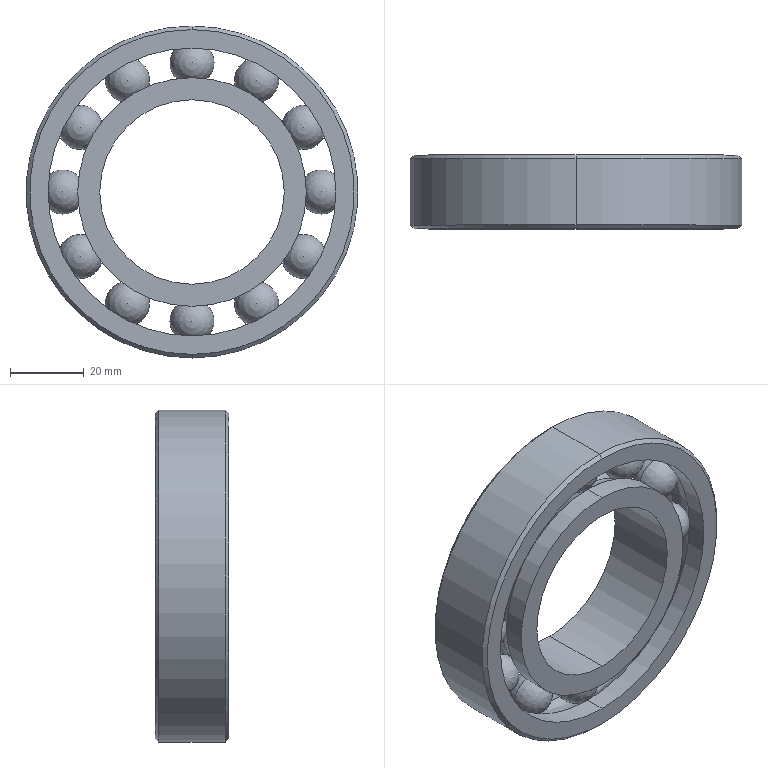Part | SolidWorks | features Revolution 13, Chamfer 1 | 14 solids | 50 faces | box 90 x 20 x 90 mm | volume 54381 mm3 | sphere 24 | cylinder 10 | torus 6 | cone 6 | plane 4 | commonest cylinder face diameters 62 x4 50 x2 78 x2 90 x2
STEP:
#1=CARTESIAN_POINT('',(0.,4.472,31.));
#2=VERTEX_POINT('',#1);
#3=CARTESIAN_POINT('',(0.,0.,29.));
#4=VERTEX_POINT('',#3);
#5=CARTESIAN_POINT('',(0.,0.,35.));
#6=DIRECTION('',(-1.,0.,0.));
#7=DIRECTION('',(0.,0.,1.));
#8=AXIS2_PLACEMENT_3D('',#5,#6,#7);
#9=CIRCLE('',#8,6.);
#10=EDGE_CURVE('',#2,#4,#9,.T.);
#11=ORIENTED_EDGE('',*,*,#10,.T.);
#12=CARTESIAN_POINT('',(0.,0.,-29.));
#13=VERTEX_POINT('',#12);
#14=CARTESIAN_POINT('',(0.,0.,0.));
#15=DIRECTION('',(0.,1.,0.));
#16=DIRECTION('',(0.,0.,1.));
#17=AXIS2_PLACEMENT_3D('',#14,#15,#16);
#18=CIRCLE('',#17,29.);
#19=EDGE_CURVE('',#4,#13,#18,.T.);
#20=ORIENTED_EDGE('',*,*,#19,.T.);
#21=CARTESIAN_POINT('',(0.,4.472,-31.));
#22=VERTEX_POINT('',#21);
#23=CARTESIAN_POINT('',(0.,0.,-35.));
#24=DIRECTION('',(1.,0.,0.));
#25=DIRECTION('',(0.,0.,-1.));
#26=AXIS2_PLACEMENT_3D('',#23,#24,#25);
#27=CIRCLE('',#26,6.);
#28=EDGE_CURVE('',#22,#13,#27,.T.);
#29=ORIENTED_EDGE('',*,*,#28,.F.);
#30=CARTESIAN_POINT('',(0.,4.472,0.));
#31=DIRECTION('',(0.,1.,0.));
#32=DIRECTION('',(0.,0.,1.));
#33=AXIS2_PLACEMENT_3D('',#30,#31,#32);
#34=CIRCLE('',#33,31.);
#35=EDGE_CURVE('',#2,#22,#34,.T.);
#36=ORIENTED_EDGE('',*,*,#35,.F.);
#37=EDGE_LOOP('',(#11,#20,#29,#36));
#38=FACE_OUTER_BOUND('',#37,.T.);
#39=CARTESIAN_POINT('',(0.,0.,0.));
#40=DIRECTION('',(0.,1.,0.));
#41=DIRECTION('',(0.,0.,1.));
#42=AXIS2_PLACEMENT_3D('',#39,#40,#41);
#43=TOROIDAL_SURFACE('',#42,35.,6.);
#44=ADVANCED_FACE('',(#38),#43,.F.);
#45=ORIENTED_EDGE('',*,*,#28,.T.);
#46=CARTESIAN_POINT('',(0.,0.,0.));
#47=DIRECTION('',(0.,1.,0.));
#48=DIRECTION('',(0.,0.,1.));
#49=AXIS2_PLACEMENT_3D('',#46,#47,#48);
#50=CIRCLE('',#49,29.);
#51=EDGE_CURVE('',#13,#4,#50,.T.);
#52=ORIENTED_EDGE('',*,*,#51,.T.);
#53=ORIENTED_EDGE('',*,*,#10,.F.);
#54=CARTESIAN_POINT('',(0.,4.472,0.));
#55=DIRECTION('',(0.,1.,0.));
#56=DIRECTION('',(0.,0.,1.));
#57=AXIS2_PLACEMENT_3D('',#54,#55,#56);
#58=CIRCLE('',#57,31.);
#59=EDGE_CURVE('',#22,#2,#58,.T.);
#60=ORIENTED_EDGE('',*,*,#59,.F.);
#61=EDGE_LOOP('',(#45,#52,#53,#60));
#62=FACE_OUTER_BOUND('',#61,.T.);
#63=CARTESIAN_POINT('',(0.,0.,0.));
#64=DIRECTION('',(0.,1.,0.));
#65=DIRECTION('',(0.,0.,1.));
#66=AXIS2_PLACEMENT_3D('',#63,#64,#65);
#67=TOROIDAL_SURFACE('',#66,35.,6.);
#68=ADVANCED_FACE('',(#62),#67,.F.);
#69=ORIENTED_EDGE('',*,*,#35,.T.);
#70=CARTESIAN_POINT('',(0.,10.,-31.));
#71=VERTEX_POINT('',#70);
#72=CARTESIAN_POINT('',(0.,0.,-31.));
#73=DIRECTION('',(0.,1.,0.));
#74=VECTOR('',#73,1000.);
#75=LINE('',#72,#74);
#76=EDGE_CURVE('',#22,#71,#75,.T.);
#77=ORIENTED_EDGE('',*,*,#76,.T.);
#78=CARTESIAN_POINT('',(0.,10.,31.));
#79=VERTEX_POINT('',#78);
#80=CARTESIAN_POINT('',(0.,10.,0.));
#81=DIRECTION('',(0.,1.,0.));
#82=DIRECTION('',(0.,0.,1.));
#83=AXIS2_PLACEMENT_3D('',#80,#81,#82);
#84=CIRCLE('',#83,31.);
#85=EDGE_CURVE('',#79,#71,#84,.T.);
#86=ORIENTED_EDGE('',*,*,#85,.F.);
#87=CARTESIAN_POINT('',(0.,0.,31.));
#88=DIRECTION('',(0.,1.,0.));
#89=VECTOR('',#88,1000.);
#90=LINE('',#87,#89);
#91=EDGE_CURVE('',#2,#79,#90,.T.);
#92=ORIENTED_EDGE('',*,*,#91,.F.);
#93=EDGE_LOOP('',(#69,#77,#86,#92));
#94=FACE_OUTER_BOUND('',#93,.T.);
#95=CARTESIAN_POINT('',(0.,0.,0.));
#96=DIRECTION('',(0.,1.,0.));
#97=DIRECTION('',(0.,0.,1.));
#98=AXIS2_PLACEMENT_3D('',#95,#96,#97);
#99=CYLINDRICAL_SURFACE('',#98,31.);
#100=ADVANCED_FACE('',(#94),#99,.T.);
#101=CARTESIAN_POINT('',(0.,-10.,-25.));
#102=VERTEX_POINT('',#101);
#103=CARTESIAN_POINT('',(0.,-10.,25.));
#104=VERTEX_POINT('',#103);
#105=CARTESIAN_POINT('',(0.,-10.,0.));
#106=DIRECTION('',(0.,1.,0.));
#107=DIRECTION('',(0.,0.,1.));
#108=AXIS2_PLACEMENT_3D('',#105,#106,#107);
#109=CIRCLE('',#108,25.);
#110=EDGE_CURVE('',#102,#104,#109,.T.);
#111=ORIENTED_EDGE('',*,*,#110,.F.);
#112=CARTESIAN_POINT('',(0.,10.,-25.));
#113=VERTEX_POINT('',#112);
#114=CARTESIAN_POINT('',(0.,0.,-25.));
#115=DIRECTION('',(0.,1.,0.));
#116=VECTOR('',#115,1000.);
#117=LINE('',#114,#116);
#118=EDGE_CURVE('',#102,#113,#117,.T.);
#119=ORIENTED_EDGE('',*,*,#118,.T.);
#120=CARTESIAN_POINT('',(0.,10.,25.));
#121=VERTEX_POINT('',#120);
#122=CARTESIAN_POINT('',(0.,10.,0.));
#123=DIRECTION('',(0.,1.,0.));
#124=DIRECTION('',(0.,0.,1.));
#125=AXIS2_PLACEMENT_3D('',#122,#123,#124);
#126=CIRCLE('',#125,25.);
#127=EDGE_CURVE('',#113,#121,#126,.T.);
#128=ORIENTED_EDGE('',*,*,#127,.T.);
#129=CARTESIAN_POINT('',(0.,0.,25.));
#130=DIRECTION('',(0.,1.,0.));
#131=VECTOR('',#130,1000.);
#132=LINE('',#129,#131);
#133=EDGE_CURVE('',#104,#121,#132,.T.);
#134=ORIENTED_EDGE('',*,*,#133,.F.);
#135=EDGE_LOOP('',(#111,#119,#128,#134));
#136=FACE_OUTER_BOUND('',#135,.T.);
#137=CARTESIAN_POINT('',(0.,0.,0.));
#138=DIRECTION('',(0.,1.,0.));
#139=DIRECTION('',(0.,0.,1.));
#140=AXIS2_PLACEMENT_3D('',#137,#138,#139);
#141=CYLINDRICAL_SURFACE('',#140,25.);
#142=ADVANCED_FACE('',(#136),#141,.F.);
#143=CARTESIAN_POINT('',(0.,-10.,31.));
#144=VERTEX_POINT('',#143);
#145=CARTESIAN_POINT('',(0.,-10.,-31.));
#146=VERTEX_POINT('',#145);
#147=CARTESIAN_POINT('',(0.,-10.,0.));
#148=DIRECTION('',(0.,1.,0.));
#149=DIRECTION('',(0.,0.,1.));
#150=AXIS2_PLACEMENT_3D('',#147,#148,#149);
#151=CIRCLE('',#150,31.);
#152=EDGE_CURVE('',#144,#146,#151,.T.);
#153=ORIENTED_EDGE('',*,*,#152,.T.);
#154=CARTESIAN_POINT('',(0.,-4.472,-31.));
#155=VERTEX_POINT('',#154);
#156=CARTESIAN_POINT('',(0.,0.,-31.));
#157=DIRECTION('',(0.,1.,0.));
#158=VECTOR('',#157,1000.);
#159=LINE('',#156,#158);
#160=EDGE_CURVE('',#146,#155,#159,.T.);
#161=ORIENTED_EDGE('',*,*,#160,.T.);
#162=CARTESIAN_POINT('',(0.,-4.472,31.));
#163=VERTEX_POINT('',#162);
#164=CARTESIAN_POINT('',(0.,-4.472,0.));
#165=DIRECTION('',(0.,1.,0.));
#166=DIRECTION('',(0.,0.,1.));
#167=AXIS2_PLACEMENT_3D('',#164,#165,#166);
#168=CIRCLE('',#167,31.);
#169=EDGE_CURVE('',#163,#155,#168,.T.);
#170=ORIENTED_EDGE('',*,*,#169,.F.);
#171=CARTESIAN_POINT('',(0.,0.,31.));
#172=DIRECTION('',(0.,1.,0.));
#173=VECTOR('',#172,1000.);
#174=LINE('',#171,#173);
#175=EDGE_CURVE('',#144,#163,#174,.T.);
#176=ORIENTED_EDGE('',*,*,#175,.F.);
#177=EDGE_LOOP('',(#153,#161,#170,#176));
#178=FACE_OUTER_BOUND('',#177,.T.);
#179=CARTESIAN_POINT('',(0.,0.,0.));
#180=DIRECTION('',(0.,1.,0.));
#181=DIRECTION('',(0.,0.,1.));
#182=AXIS2_PLACEMENT_3D('',#179,#180,#181);
#183=CYLINDRICAL_SURFACE('',#182,31.);
#184=ADVANCED_FACE('',(#178),#183,.T.);
#185=ORIENTED_EDGE('',*,*,#51,.F.);
#186=CARTESIAN_POINT('',(0.,0.,-35.));
#187=DIRECTION('',(1.,0.,0.));
#188=DIRECTION('',(0.,0.,-1.));
#189=AXIS2_PLACEMENT_3D('',#186,#187,#188);
#190=CIRCLE('',#189,6.);
#191=EDGE_CURVE('',#13,#155,#190,.T.);
#192=ORIENTED_EDGE('',*,*,#191,.T.);
#193=CARTESIAN_POINT('',(0.,-4.472,0.));
#194=DIRECTION('',(0.,1.,0.));
#195=DIRECTION('',(0.,0.,1.));
#196=AXIS2_PLACEMENT_3D('',#193,#194,#195);
#197=CIRCLE('',#196,31.);
#198=EDGE_CURVE('',#155,#163,#197,.T.);
#199=ORIENTED_EDGE('',*,*,#198,.T.);
#200=CARTESIAN_POINT('',(0.,0.,35.));
#201=DIRECTION('',(-1.,0.,0.));
#202=DIRECTION('',(0.,0.,1.));
#203=AXIS2_PLACEMENT_3D('',#200,#201,#202);
#204=CIRCLE('',#203,6.);
#205=EDGE_CURVE('',#4,#163,#204,.T.);
#206=ORIENTED_EDGE('',*,*,#205,.F.);
#207=EDGE_LOOP('',(#185,#192,#199,#206));
#208=FACE_OUTER_BOUND('',#207,.T.);
#209=CARTESIAN_POINT('',(0.,0.,0.));
#210=DIRECTION('',(0.,1.,0.));
#211=DIRECTION('',(0.,0.,1.));
#212=AXIS2_PLACEMENT_3D('',#209,#210,#211);
#213=TOROIDAL_SURFACE('',#212,35.,6.);
#214=ADVANCED_FACE('',(#208),#213,.F.);
#215=ORIENTED_EDGE('',*,*,#19,.F.);
#216=ORIENTED_EDGE('',*,*,#205,.T.);
#217=ORIENTED_EDGE('',*,*,#169,.T.);
#218=ORIENTED_EDGE('',*,*,#191,.F.);
#219=EDGE_LOOP('',(#215,#216,#217,#218));
#220=FACE_OUTER_BOUND('',#219,.T.);
#221=CARTESIAN_POINT('',(0.,0.,0.));
#222=DIRECTION('',(0.,1.,0.));
#223=DIRECTION('',(0.,0.,1.));
#224=AXIS2_PLACEMENT_3D('',#221,#222,#223);
#225=TOROIDAL_SURFACE('',#224,35.,6.);
#226=ADVANCED_FACE('',(#220),#225,.F.);
#227=ORIENTED_EDGE('',*,*,#160,.F.);
#228=CARTESIAN_POINT('',(0.,-10.,0.));
#229=DIRECTION('',(0.,1.,0.));
#230=DIRECTION('',(0.,0.,1.));
#231=AXIS2_PLACEMENT_3D('',#228,#229,#230);
#232=CIRCLE('',#231,31.);
#233=EDGE_CURVE('',#146,#144,#232,.T.);
#234=ORIENTED_EDGE('',*,*,#233,.T.);
#235=ORIENTED_EDGE('',*,*,#175,.T.);
#236=ORIENTED_EDGE('',*,*,#198,.F.);
#237=EDGE_LOOP('',(#227,#234,#235,#236));
#238=FACE_OUTER_BOUND('',#237,.T.);
#239=CARTESIAN_POINT('',(0.,0.,0.));
#240=DIRECTION('',(0.,1.,0.));
#241=DIRECTION('',(0.,0.,1.));
#242=AXIS2_PLACEMENT_3D('',#239,#240,#241);
#243=CYLINDRICAL_SURFACE('',#242,31.);
#244=ADVANCED_FACE('',(#238),#243,.T.);
#245=CARTESIAN_POINT('',(0.,-10.,0.));
#246=DIRECTION('',(0.,1.,0.));
#247=DIRECTION('',(0.,0.,1.));
#248=AXIS2_PLACEMENT_3D('',#245,#246,#247);
#249=CIRCLE('',#248,25.);
#250=EDGE_CURVE('',#104,#102,#249,.T.);
#251=ORIENTED_EDGE('',*,*,#250,.T.);
#252=ORIENTED_EDGE('',*,*,#110,.T.);
#253=EDGE_LOOP('',(#251,#252));
#254=FACE_BOUND('',#253,.T.);
#255=ORIENTED_EDGE('',*,*,#152,.F.);
#256=ORIENTED_EDGE('',*,*,#233,.F.);
#257=EDGE_LOOP('',(#255,#256));
#258=FACE_OUTER_BOUND('',#257,.T.);
#259=CARTESIAN_POINT('',(-25.,-10.,0.));
#260=DIRECTION('',(0.,-1.,0.));
#261=DIRECTION('',(0.,0.,-1.));
#262=AXIS2_PLACEMENT_3D('',#259,#260,#261);
#263=PLANE('',#262);
#264=ADVANCED_FACE('',(#254,#258),#263,.T.);
#265=ORIENTED_EDGE('',*,*,#118,.F.);
#266=ORIENTED_EDGE('',*,*,#250,.F.);
#267=ORIENTED_EDGE('',*,*,#133,.T.);
#268=CARTESIAN_POINT('',(0.,10.,0.));
#269=DIRECTION('',(0.,1.,0.));
#270=DIRECTION('',(0.,0.,1.));
#271=AXIS2_PLACEMENT_3D('',#268,#269,#270);
#272=CIRCLE('',#271,25.);
#273=EDGE_CURVE('',#121,#113,#272,.T.);
#274=ORIENTED_EDGE('',*,*,#273,.T.);
#275=EDGE_LOOP('',(#265,#266,#267,#274));
#276=FACE_OUTER_BOUND('',#275,.T.);
#277=CARTESIAN_POINT('',(0.,0.,0.));
#278=DIRECTION('',(0.,1.,0.));
#279=DIRECTION('',(0.,0.,1.));
#280=AXIS2_PLACEMENT_3D('',#277,#278,#279);
#281=CYLINDRICAL_SURFACE('',#280,25.);
#282=ADVANCED_FACE('',(#276),#281,.F.);
#283=ORIENTED_EDGE('',*,*,#85,.T.);
#284=CARTESIAN_POINT('',(0.,10.,0.));
#285=DIRECTION('',(0.,1.,0.));
#286=DIRECTION('',(0.,0.,1.));
#287=AXIS2_PLACEMENT_3D('',#284,#285,#286);
#288=CIRCLE('',#287,31.);
#289=EDGE_CURVE('',#71,#79,#288,.T.);
#290=ORIENTED_EDGE('',*,*,#289,.T.);
#291=EDGE_LOOP('',(#283,#290));
#292=FACE_OUTER_BOUND('',#291,.T.);
#293=ORIENTED_EDGE('',*,*,#273,.F.);
#294=ORIENTED_EDGE('',*,*,#127,.F.);
#295=EDGE_LOOP('',(#293,#294));
#296=FACE_BOUND('',#295,.T.);
#297=CARTESIAN_POINT('',(-25.,10.,0.));
#298=DIRECTION('',(0.,1.,0.));
#299=DIRECTION('',(0.,0.,1.));
#300=AXIS2_PLACEMENT_3D('',#297,#298,#299);
#301=PLANE('',#300);
#302=ADVANCED_FACE('',(#292,#296),#301,.T.);
#303=ORIENTED_EDGE('',*,*,#76,.F.);
#304=ORIENTED_EDGE('',*,*,#59,.T.);
#305=ORIENTED_EDGE('',*,*,#91,.T.);
#306=ORIENTED_EDGE('',*,*,#289,.F.);
#307=EDGE_LOOP('',(#303,#304,#305,#306));
#308=FACE_OUTER_BOUND('',#307,.T.);
#309=CARTESIAN_POINT('',(0.,0.,0.));
#310=DIRECTION('',(0.,1.,0.));
#311=DIRECTION('',(0.,0.,1.));
#312=AXIS2_PLACEMENT_3D('',#309,#310,#311);
#313=CYLINDRICAL_SURFACE('',#312,31.);
#314=ADVANCED_FACE('',(#308),#313,.T.);
#315=CLOSED_SHELL('',(#44,#68,#100,#142,#184,#214,#226,#244,#264,#282,#302,#314));
#316=MANIFOLD_SOLID_BREP('',#315);
#317=CARTESIAN_POINT('',(0.,-10.,-44.));
#318=VERTEX_POINT('',#317);
#319=CARTESIAN_POINT('',(0.,-10.,44.));
#320=VERTEX_POINT('',#319);
#321=CARTESIAN_POINT('',(0.,-10.,0.));
#322=DIRECTION('',(0.,-1.,0.));
#323=DIRECTION('',(0.,0.,-1.));
#324=AXIS2_PLACEMENT_3D('',#321,#322,#323);
#325=CIRCLE('',#324,44.);
#326=EDGE_CURVE('',#318,#320,#325,.T.);
#327=ORIENTED_EDGE('',*,*,#326,.F.);
#328=CARTESIAN_POINT('',(0.,-9.,-45.));
#329=VERTEX_POINT('',#328);
#330=CARTESIAN_POINT('',(0.,-9.,-45.));
#331=DIRECTION('',(0.,0.7071,-0.7071));
#332=VECTOR('',#331,1000.);
#333=LINE('',#330,#332);
#334=EDGE_CURVE('',#318,#329,#333,.T.);
#335=ORIENTED_EDGE('',*,*,#334,.T.);
#336=CARTESIAN_POINT('',(0.,-9.,45.));
#337=VERTEX_POINT('',#336);
#338=CARTESIAN_POINT('',(0.,-9.,0.));
#339=DIRECTION('',(0.,1.,0.));
#340=DIRECTION('',(0.,0.,-1.));
#341=AXIS2_PLACEMENT_3D('',#338,#339,#340);
#342=CIRCLE('',#341,45.);
#343=EDGE_CURVE('',#337,#329,#342,.T.);
#344=ORIENTED_EDGE('',*,*,#343,.F.);
#345=CARTESIAN_POINT('',(0.,-9.,45.));
#346=DIRECTION('',(0.,0.7071,0.7071));
#347=VECTOR('',#346,1000.);
#348=LINE('',#345,#347);
#349=EDGE_CURVE('',#320,#337,#348,.T.);
#350=ORIENTED_EDGE('',*,*,#349,.F.);
#351=EDGE_LOOP('',(#327,#335,#344,#350));
#352=FACE_OUTER_BOUND('',#351,.T.);
#353=CARTESIAN_POINT('',(0.,-9.,0.));
#354=DIRECTION('',(0.,1.,0.));
#355=DIRECTION('',(0.,0.,1.));
#356=AXIS2_PLACEMENT_3D('',#353,#354,#355);
#357=CONICAL_SURFACE('',#356,45.,0.7854);
#358=ADVANCED_FACE('',(#352),#357,.T.);
#359=CARTESIAN_POINT('',(0.,10.,44.));
#360=VERTEX_POINT('',#359);
#361=CARTESIAN_POINT('',(0.,10.,-44.));
#362=VERTEX_POINT('',#361);
#363=CARTESIAN_POINT('',(0.,10.,0.));
#364=DIRECTION('',(0.,1.,0.));
#365=DIRECTION('',(0.,0.,1.));
#366=AXIS2_PLACEMENT_3D('',#363,#364,#365);
#367=CIRCLE('',#366,44.);
#368=EDGE_CURVE('',#360,#362,#367,.T.);
#369=ORIENTED_EDGE('',*,*,#368,.F.);
#370=CARTESIAN_POINT('',(0.,9.,45.));
#371=VERTEX_POINT('',#370);
#372=CARTESIAN_POINT('',(0.,10.,44.));
#373=DIRECTION('',(0.,-0.7071,0.7071));
#374=VECTOR('',#373,1000.);
#375=LINE('',#372,#374);
#376=EDGE_CURVE('',#360,#371,#375,.T.);
#377=ORIENTED_EDGE('',*,*,#376,.T.);
#378=CARTESIAN_POINT('',(0.,9.,-45.));
#379=VERTEX_POINT('',#378);
#380=CARTESIAN_POINT('',(0.,9.,0.));
#381=DIRECTION('',(0.,-1.,0.));
#382=DIRECTION('',(0.,0.,1.));
#383=AXIS2_PLACEMENT_3D('',#380,#381,#382);
#384=CIRCLE('',#383,45.);
#385=EDGE_CURVE('',#379,#371,#384,.T.);
#386=ORIENTED_EDGE('',*,*,#385,.F.);
#387=CARTESIAN_POINT('',(0.,10.,-44.));
#388=DIRECTION('',(0.,-0.7071,-0.7071));
#389=VECTOR('',#388,1000.);
#390=LINE('',#387,#389);
#391=EDGE_CURVE('',#362,#379,#390,.T.);
#392=ORIENTED_EDGE('',*,*,#391,.F.);
#393=EDGE_LOOP('',(#369,#377,#386,#392));
#394=FACE_OUTER_BOUND('',#393,.T.);
#395=CARTESIAN_POINT('',(0.,10.,0.));
#396=DIRECTION('',(0.,-1.,0.));
#397=DIRECTION('',(0.,0.,-1.));
#398=AXIS2_PLACEMENT_3D('',#395,#396,#397);
#399=CONICAL_SURFACE('',#398,44.,0.7854);
#400=ADVANCED_FACE('',(#394),#399,.T.);
#401=CARTESIAN_POINT('',(0.,-10.,-39.));
#402=VERTEX_POINT('',#401);
#403=CARTESIAN_POINT('',(0.,-10.,39.));
#404=VERTEX_POINT('',#403);
#405=CARTESIAN_POINT('',(0.,-10.,0.));
#406=DIRECTION('',(0.,1.,0.));
#407=DIRECTION('',(0.,0.,1.));
#408=AXIS2_PLACEMENT_3D('',#405,#406,#407);
#409=CIRCLE('',#408,39.);
#410=EDGE_CURVE('',#402,#404,#409,.T.);
#411=ORIENTED_EDGE('',*,*,#410,.F.);
#412=CARTESIAN_POINT('',(0.,-4.472,-39.));
#413=VERTEX_POINT('',#412);
#414=CARTESIAN_POINT('',(0.,0.,-39.));
#415=DIRECTION('',(0.,1.,0.));
#416=VECTOR('',#415,1000.);
#417=LINE('',#414,#416);
#418=EDGE_CURVE('',#402,#413,#417,.T.);
#419=ORIENTED_EDGE('',*,*,#418,.T.);
#420=CARTESIAN_POINT('',(0.,-4.472,39.));
#421=VERTEX_POINT('',#420);
#422=CARTESIAN_POINT('',(0.,-4.472,0.));
#423=DIRECTION('',(0.,1.,0.));
#424=DIRECTION('',(0.,0.,1.));
#425=AXIS2_PLACEMENT_3D('',#422,#423,#424);
#426=CIRCLE('',#425,39.);
#427=EDGE_CURVE('',#413,#421,#426,.T.);
#428=ORIENTED_EDGE('',*,*,#427,.T.);
#429=CARTESIAN_POINT('',(0.,0.,39.));
#430=DIRECTION('',(0.,1.,0.));
#431=VECTOR('',#430,1000.);
#432=LINE('',#429,#431);
#433=EDGE_CURVE('',#404,#421,#432,.T.);
#434=ORIENTED_EDGE('',*,*,#433,.F.);
#435=EDGE_LOOP('',(#411,#419,#428,#434));
#436=FACE_OUTER_BOUND('',#435,.T.);
#437=CARTESIAN_POINT('',(0.,0.,0.));
#438=DIRECTION('',(0.,1.,0.));
#439=DIRECTION('',(0.,0.,1.));
#440=AXIS2_PLACEMENT_3D('',#437,#438,#439);
#441=CYLINDRICAL_SURFACE('',#440,39.);
#442=ADVANCED_FACE('',(#436),#441,.F.);
#443=ORIENTED_EDGE('',*,*,#343,.T.);
#444=CARTESIAN_POINT('',(0.,0.,-45.));
#445=DIRECTION('',(0.,1.,0.));
#446=VECTOR('',#445,1000.);
#447=LINE('',#444,#446);
#448=EDGE_CURVE('',#329,#379,#447,.T.);
#449=ORIENTED_EDGE('',*,*,#448,.T.);
#450=ORIENTED_EDGE('',*,*,#385,.T.);
#451=CARTESIAN_POINT('',(0.,0.,45.));
#452=DIRECTION('',(0.,1.,0.));
#453=VECTOR('',#452,1000.);
#454=LINE('',#451,#453);
#455=EDGE_CURVE('',#337,#371,#454,.T.);
#456=ORIENTED_EDGE('',*,*,#455,.F.);
#457=EDGE_LOOP('',(#443,#449,#450,#456));
#458=FACE_OUTER_BOUND('',#457,.T.);
#459=CARTESIAN_POINT('',(0.,0.,0.));
#460=DIRECTION('',(0.,1.,0.));
#461=DIRECTION('',(0.,0.,1.));
#462=AXIS2_PLACEMENT_3D('',#459,#460,#461);
#463=CYLINDRICAL_SURFACE('',#462,45.);
#464=ADVANCED_FACE('',(#458),#463,.T.);
#465=CARTESIAN_POINT('',(0.,3.,-40.196));
#466=VERTEX_POINT('',#465);
#467=CARTESIAN_POINT('',(0.,3.,40.196));
#468=VERTEX_POINT('',#467);
#469=CARTESIAN_POINT('',(0.,3.,0.));
#470=DIRECTION('',(0.,1.,0.));
#471=DIRECTION('',(0.,0.,1.));
#472=AXIS2_PLACEMENT_3D('',#469,#470,#471);
#473=CIRCLE('',#472,40.196);
#474=EDGE_CURVE('',#466,#468,#473,.T.);
#475=ORIENTED_EDGE('',*,*,#474,.F.);
#476=CARTESIAN_POINT('',(0.,10.,-42.072));
#477=VERTEX_POINT('',#476);
#478=CARTESIAN_POINT('',(0.,3.,-40.196));
#479=DIRECTION('',(0.,0.9659,-0.2588));
#480=VECTOR('',#479,1000.);
#481=LINE('',#478,#480);
#482=EDGE_CURVE('',#466,#477,#481,.T.);
#483=ORIENTED_EDGE('',*,*,#482,.T.);
#484=CARTESIAN_POINT('',(0.,10.,42.072));
#485=VERTEX_POINT('',#484);
#486=CARTESIAN_POINT('',(0.,10.,0.));
#487=DIRECTION('',(0.,1.,0.));
#488=DIRECTION('',(0.,0.,1.));
#489=AXIS2_PLACEMENT_3D('',#486,#487,#488);
#490=CIRCLE('',#489,42.072);
#491=EDGE_CURVE('',#477,#485,#490,.T.);
#492=ORIENTED_EDGE('',*,*,#491,.T.);
#493=CARTESIAN_POINT('',(0.,3.,40.196));
#494=DIRECTION('',(0.,0.9659,0.2588));
#495=VECTOR('',#494,1000.);
#496=LINE('',#493,#495);
#497=EDGE_CURVE('',#468,#485,#496,.T.);
#498=ORIENTED_EDGE('',*,*,#497,.F.);
#499=EDGE_LOOP('',(#475,#483,#492,#498));
#500=FACE_OUTER_BOUND('',#499,.T.);
#501=CARTESIAN_POINT('',(0.,3.,0.));
#502=DIRECTION('',(0.,1.,0.));
#503=DIRECTION('',(0.,0.,1.));
#504=AXIS2_PLACEMENT_3D('',#501,#502,#503);
#505=CONICAL_SURFACE('',#504,40.196,0.2618);
#506=ADVANCED_FACE('',(#500),#505,.F.);
#507=ORIENTED_EDGE('',*,*,#427,.F.);
#508=CARTESIAN_POINT('',(0.,0.,-35.));
#509=DIRECTION('',(1.,0.,0.));
#510=DIRECTION('',(0.,0.,-1.));
#511=AXIS2_PLACEMENT_3D('',#508,#509,#510);
#512=CIRCLE('',#511,6.);
#513=EDGE_CURVE('',#413,#466,#512,.T.);
#514=ORIENTED_EDGE('',*,*,#513,.T.);
#515=ORIENTED_EDGE('',*,*,#474,.T.);
#516=CARTESIAN_POINT('',(0.,0.,35.));
#517=DIRECTION('',(-1.,0.,0.));
#518=DIRECTION('',(0.,0.,1.));
#519=AXIS2_PLACEMENT_3D('',#516,#517,#518);
#520=CIRCLE('',#519,6.);
#521=EDGE_CURVE('',#421,#468,#520,.T.);
#522=ORIENTED_EDGE('',*,*,#521,.F.);
#523=EDGE_LOOP('',(#507,#514,#515,#522));
#524=FACE_OUTER_BOUND('',#523,.T.);
#525=CARTESIAN_POINT('',(0.,0.,0.));
#526=DIRECTION('',(0.,1.,0.));
#527=DIRECTION('',(0.,0.,1.));
#528=AXIS2_PLACEMENT_3D('',#525,#526,#527);
#529=TOROIDAL_SURFACE('',#528,35.,6.);
#530=ADVANCED_FACE('',(#524),#529,.F.);
#531=ORIENTED_EDGE('',*,*,#513,.F.);
#532=CARTESIAN_POINT('',(0.,-4.472,0.));
#533=DIRECTION('',(0.,1.,0.));
#534=DIRECTION('',(0.,0.,1.));
#535=AXIS2_PLACEMENT_3D('',#532,#533,#534);
#536=CIRCLE('',#535,39.);
#537=EDGE_CURVE('',#421,#413,#536,.T.);
#538=ORIENTED_EDGE('',*,*,#537,.F.);
#539=ORIENTED_EDGE('',*,*,#521,.T.);
#540=CARTESIAN_POINT('',(0.,3.,0.));
#541=DIRECTION('',(0.,1.,0.));
#542=DIRECTION('',(0.,0.,1.));
#543=AXIS2_PLACEMENT_3D('',#540,#541,#542);
#544=CIRCLE('',#543,40.196);
#545=EDGE_CURVE('',#468,#466,#544,.T.);
#546=ORIENTED_EDGE('',*,*,#545,.T.);
#547=EDGE_LOOP('',(#531,#538,#539,#546));
#548=FACE_OUTER_BOUND('',#547,.T.);
#549=CARTESIAN_POINT('',(0.,0.,0.));
#550=DIRECTION('',(0.,1.,0.));
#551=DIRECTION('',(0.,0.,1.));
#552=AXIS2_PLACEMENT_3D('',#549,#550,#551);
#553=TOROIDAL_SURFACE('',#552,35.,6.);
#554=ADVANCED_FACE('',(#548),#553,.F.);
#555=ORIENTED_EDGE('',*,*,#482,.F.);
#556=ORIENTED_EDGE('',*,*,#545,.F.);
#557=ORIENTED_EDGE('',*,*,#497,.T.);
#558=CARTESIAN_POINT('',(0.,10.,0.));
#559=DIRECTION('',(0.,1.,0.));
#560=DIRECTION('',(0.,0.,1.));
#561=AXIS2_PLACEMENT_3D('',#558,#559,#560);
#562=CIRCLE('',#561,42.072);
#563=EDGE_CURVE('',#485,#477,#562,.T.);
#564=ORIENTED_EDGE('',*,*,#563,.T.);
#565=EDGE_LOOP('',(#555,#556,#557,#564));
#566=FACE_OUTER_BOUND('',#565,.T.);
#567=CARTESIAN_POINT('',(0.,3.,0.));
#568=DIRECTION('',(0.,1.,0.));
#569=DIRECTION('',(0.,0.,1.));
#570=AXIS2_PLACEMENT_3D('',#567,#568,#569);
#571=CONICAL_SURFACE('',#570,40.196,0.2618);
#572=ADVANCED_FACE('',(#566),#571,.F.);
#573=CARTESIAN_POINT('',(0.,10.,0.));
#574=DIRECTION('',(0.,1.,0.));
#575=DIRECTION('',(0.,0.,1.));
#576=AXIS2_PLACEMENT_3D('',#573,#574,#575);
#577=CIRCLE('',#576,44.);
#578=EDGE_CURVE('',#362,#360,#577,.T.);
#579=ORIENTED_EDGE('',*,*,#578,.T.);
#580=ORIENTED_EDGE('',*,*,#368,.T.);
#581=EDGE_LOOP('',(#579,#580));
#582=FACE_OUTER_BOUND('',#581,.T.);
#583=ORIENTED_EDGE('',*,*,#563,.F.);
#584=ORIENTED_EDGE('',*,*,#491,.F.);
#585=EDGE_LOOP('',(#583,#584));
#586=FACE_BOUND('',#585,.T.);
#587=CARTESIAN_POINT('',(-42.072,10.,0.));
#588=DIRECTION('',(0.,1.,0.));
#589=DIRECTION('',(0.,0.,1.));
#590=AXIS2_PLACEMENT_3D('',#587,#588,#589);
#591=PLANE('',#590);
#592=ADVANCED_FACE('',(#582,#586),#591,.T.);
#593=ORIENTED_EDGE('',*,*,#448,.F.);
#594=CARTESIAN_POINT('',(0.,-9.,0.));
#595=DIRECTION('',(0.,1.,0.));
#596=DIRECTION('',(0.,0.,-1.));
#597=AXIS2_PLACEMENT_3D('',#594,#595,#596);
#598=CIRCLE('',#597,45.);
#599=EDGE_CURVE('',#329,#337,#598,.T.);
#600=ORIENTED_EDGE('',*,*,#599,.T.);
#601=ORIENTED_EDGE('',*,*,#455,.T.);
#602=CARTESIAN_POINT('',(0.,9.,0.));
#603=DIRECTION('',(0.,-1.,0.));
#604=DIRECTION('',(0.,0.,1.));
#605=AXIS2_PLACEMENT_3D('',#602,#603,#604);
#606=CIRCLE('',#605,45.);
#607=EDGE_CURVE('',#371,#379,#606,.T.);
#608=ORIENTED_EDGE('',*,*,#607,.T.);
#609=EDGE_LOOP('',(#593,#600,#601,#608));
#610=FACE_OUTER_BOUND('',#609,.T.);
#611=CARTESIAN_POINT('',(0.,0.,0.));
#612=DIRECTION('',(0.,1.,0.));
#613=DIRECTION('',(0.,0.,1.));
#614=AXIS2_PLACEMENT_3D('',#611,#612,#613);
#615=CYLINDRICAL_SURFACE('',#614,45.);
#616=ADVANCED_FACE('',(#610),#615,.T.);
#617=CARTESIAN_POINT('',(0.,-10.,0.));
#618=DIRECTION('',(0.,-1.,0.));
#619=DIRECTION('',(0.,0.,-1.));
#620=AXIS2_PLACEMENT_3D('',#617,#618,#619);
#621=CIRCLE('',#620,44.);
#622=EDGE_CURVE('',#320,#318,#621,.T.);
#623=ORIENTED_EDGE('',*,*,#622,.T.);
#624=ORIENTED_EDGE('',*,*,#326,.T.);
#625=EDGE_LOOP('',(#623,#624));
#626=FACE_OUTER_BOUND('',#625,.T.);
#627=CARTESIAN_POINT('',(0.,-10.,0.));
#628=DIRECTION('',(0.,1.,0.));
#629=DIRECTION('',(0.,0.,1.));
#630=AXIS2_PLACEMENT_3D('',#627,#628,#629);
#631=CIRCLE('',#630,39.);
#632=EDGE_CURVE('',#404,#402,#631,.T.);
#633=ORIENTED_EDGE('',*,*,#632,.T.);
#634=ORIENTED_EDGE('',*,*,#410,.T.);
#635=EDGE_LOOP('',(#633,#634));
#636=FACE_BOUND('',#635,.T.);
#637=CARTESIAN_POINT('',(-39.,-10.,0.));
#638=DIRECTION('',(0.,-1.,0.));
#639=DIRECTION('',(0.,0.,-1.));
#640=AXIS2_PLACEMENT_3D('',#637,#638,#639);
#641=PLANE('',#640);
#642=ADVANCED_FACE('',(#626,#636),#641,.T.);
#643=ORIENTED_EDGE('',*,*,#418,.F.);
#644=ORIENTED_EDGE('',*,*,#632,.F.);
#645=ORIENTED_EDGE('',*,*,#433,.T.);
#646=ORIENTED_EDGE('',*,*,#537,.T.);
#647=EDGE_LOOP('',(#643,#644,#645,#646));
#648=FACE_OUTER_BOUND('',#647,.T.);
#649=CARTESIAN_POINT('',(0.,0.,0.));
#650=DIRECTION('',(0.,1.,0.));
#651=DIRECTION('',(0.,0.,1.));
#652=AXIS2_PLACEMENT_3D('',#649,#650,#651);
#653=CYLINDRICAL_SURFACE('',#652,39.);
#654=ADVANCED_FACE('',(#648),#653,.F.);
#655=ORIENTED_EDGE('',*,*,#376,.F.);
#656=ORIENTED_EDGE('',*,*,#578,.F.);
#657=ORIENTED_EDGE('',*,*,#391,.T.);
#658=ORIENTED_EDGE('',*,*,#607,.F.);
#659=EDGE_LOOP('',(#655,#656,#657,#658));
#660=FACE_OUTER_BOUND('',#659,.T.);
#661=CARTESIAN_POINT('',(0.,10.,0.));
#662=DIRECTION('',(0.,-1.,0.));
#663=DIRECTION('',(0.,0.,-1.));
#664=AXIS2_PLACEMENT_3D('',#661,#662,#663);
#665=CONICAL_SURFACE('',#664,44.,0.7854);
#666=ADVANCED_FACE('',(#660),#665,.T.);
#667=ORIENTED_EDGE('',*,*,#334,.F.);
#668=ORIENTED_EDGE('',*,*,#622,.F.);
#669=ORIENTED_EDGE('',*,*,#349,.T.);
#670=ORIENTED_EDGE('',*,*,#599,.F.);
#671=EDGE_LOOP('',(#667,#668,#669,#670));
#672=FACE_OUTER_BOUND('',#671,.T.);
#673=CARTESIAN_POINT('',(0.,-9.,0.));
#674=DIRECTION('',(0.,1.,0.));
#675=DIRECTION('',(0.,0.,1.));
#676=AXIS2_PLACEMENT_3D('',#673,#674,#675);
#677=CONICAL_SURFACE('',#676,45.,0.7854);
#678=ADVANCED_FACE('',(#672),#677,.T.);
#679=CLOSED_SHELL('',(#358,#400,#442,#464,#506,#530,#554,#572,#592,#616,#642,#654,#666,#678));
#680=MANIFOLD_SOLID_BREP('',#679);
#681=CARTESIAN_POINT('',(0.,0.,-41.));
#682=VERTEX_POINT('',#681);
#683=CARTESIAN_POINT('',(0.,0.,-29.));
#684=VERTEX_POINT('',#683);
#685=CARTESIAN_POINT('',(0.,0.,-35.));
#686=DIRECTION('',(0.,1.,0.));
#687=DIRECTION('',(0.,0.,1.));
#688=AXIS2_PLACEMENT_3D('',#685,#686,#687);
#689=CIRCLE('',#688,6.);
#690=EDGE_CURVE('',#682,#684,#689,.T.);
#691=ORIENTED_EDGE('',*,*,#690,.F.);
#692=CARTESIAN_POINT('',(0.,0.,-35.));
#693=DIRECTION('',(0.,-1.,0.));
#694=DIRECTION('',(1.,0.,0.));
#695=AXIS2_PLACEMENT_3D('',#692,#693,#694);
#696=CIRCLE('',#695,6.);
#697=EDGE_CURVE('',#682,#684,#696,.T.);
#698=ORIENTED_EDGE('',*,*,#697,.T.);
#699=EDGE_LOOP('',(#691,#698));
#700=FACE_OUTER_BOUND('',#699,.T.);
#701=CARTESIAN_POINT('',(0.,0.,-35.));
#702=DIRECTION('',(0.,-1.,0.));
#703=DIRECTION('',(-1.,0.,0.));
#704=AXIS2_PLACEMENT_3D('',#701,#702,#703);
#705=SPHERICAL_SURFACE('',#704,6.);
#706=ADVANCED_FACE('',(#700),#705,.T.);
#707=ORIENTED_EDGE('',*,*,#697,.F.);
#708=ORIENTED_EDGE('',*,*,#690,.T.);
#709=EDGE_LOOP('',(#707,#708));
#710=FACE_OUTER_BOUND('',#709,.T.);
#711=CARTESIAN_POINT('',(0.,0.,-35.));
#712=DIRECTION('',(0.,-1.,0.));
#713=DIRECTION('',(-1.,0.,0.));
#714=AXIS2_PLACEMENT_3D('',#711,#712,#713);
#715=SPHERICAL_SURFACE('',#714,6.);
#716=ADVANCED_FACE('',(#710),#715,.T.);
#717=CLOSED_SHELL('',(#706,#716));
#718=MANIFOLD_SOLID_BREP('',#717);
#719=CARTESIAN_POINT('',(-20.5,0.,-35.507));
#720=VERTEX_POINT('',#719);
#721=CARTESIAN_POINT('',(-14.5,0.,-25.115));
#722=VERTEX_POINT('',#721);
#723=CARTESIAN_POINT('',(-17.5,0.,-30.311));
#724=DIRECTION('',(0.,-1.,0.));
#725=DIRECTION('',(0.,0.,-1.));
#726=AXIS2_PLACEMENT_3D('',#723,#724,#725);
#727=CIRCLE('',#726,6.);
#728=EDGE_CURVE('',#720,#722,#727,.T.);
#729=ORIENTED_EDGE('',*,*,#728,.F.);
#730=CARTESIAN_POINT('',(-17.5,0.,-30.311));
#731=DIRECTION('',(0.,1.,0.));
#732=DIRECTION('',(-1.,0.,0.));
#733=AXIS2_PLACEMENT_3D('',#730,#731,#732);
#734=CIRCLE('',#733,6.);
#735=EDGE_CURVE('',#720,#722,#734,.T.);
#736=ORIENTED_EDGE('',*,*,#735,.T.);
#737=EDGE_LOOP('',(#729,#736));
#738=FACE_OUTER_BOUND('',#737,.T.);
#739=CARTESIAN_POINT('',(-17.5,0.,-30.311));
#740=DIRECTION('',(0.,1.,0.));
#741=DIRECTION('',(0.866,0.,-0.5));
#742=AXIS2_PLACEMENT_3D('',#739,#740,#741);
#743=SPHERICAL_SURFACE('',#742,6.);
#744=ADVANCED_FACE('',(#738),#743,.T.);
#745=ORIENTED_EDGE('',*,*,#735,.F.);
#746=ORIENTED_EDGE('',*,*,#728,.T.);
#747=EDGE_LOOP('',(#745,#746));
#748=FACE_OUTER_BOUND('',#747,.T.);
#749=CARTESIAN_POINT('',(-17.5,0.,-30.311));
#750=DIRECTION('',(0.,1.,0.));
#751=DIRECTION('',(0.866,0.,-0.5));
#752=AXIS2_PLACEMENT_3D('',#749,#750,#751);
#753=SPHERICAL_SURFACE('',#752,6.);
#754=ADVANCED_FACE('',(#748),#753,.T.);
#755=CLOSED_SHELL('',(#744,#754));
#756=MANIFOLD_SOLID_BREP('',#755);
#757=CARTESIAN_POINT('',(-35.507,0.,-20.5));
#758=VERTEX_POINT('',#757);
#759=CARTESIAN_POINT('',(-25.115,0.,-14.5));
#760=VERTEX_POINT('',#759);
#761=CARTESIAN_POINT('',(-30.311,0.,-17.5));
#762=DIRECTION('',(0.,1.,0.));
#763=DIRECTION('',(0.,0.,1.));
#764=AXIS2_PLACEMENT_3D('',#761,#762,#763);
#765=CIRCLE('',#764,6.);
#766=EDGE_CURVE('',#758,#760,#765,.T.);
#767=ORIENTED_EDGE('',*,*,#766,.F.);
#768=CARTESIAN_POINT('',(-30.311,0.,-17.5));
#769=DIRECTION('',(0.,-1.,0.));
#770=DIRECTION('',(0.,0.,-1.));
#771=AXIS2_PLACEMENT_3D('',#768,#769,#770);
#772=CIRCLE('',#771,6.);
#773=EDGE_CURVE('',#758,#760,#772,.T.);
#774=ORIENTED_EDGE('',*,*,#773,.T.);
#775=EDGE_LOOP('',(#767,#774));
#776=FACE_OUTER_BOUND('',#775,.T.);
#777=CARTESIAN_POINT('',(-30.311,0.,-17.5));
#778=DIRECTION('',(0.,-1.,0.));
#779=DIRECTION('',(-0.5,0.,0.866));
#780=AXIS2_PLACEMENT_3D('',#777,#778,#779);
#781=SPHERICAL_SURFACE('',#780,6.);
#782=ADVANCED_FACE('',(#776),#781,.T.);
#783=ORIENTED_EDGE('',*,*,#773,.F.);
#784=ORIENTED_EDGE('',*,*,#766,.T.);
#785=EDGE_LOOP('',(#783,#784));
#786=FACE_OUTER_BOUND('',#785,.T.);
#787=CARTESIAN_POINT('',(-30.311,0.,-17.5));
#788=DIRECTION('',(0.,-1.,0.));
#789=DIRECTION('',(-0.5,0.,0.866));
#790=AXIS2_PLACEMENT_3D('',#787,#788,#789);
#791=SPHERICAL_SURFACE('',#790,6.);
#792=ADVANCED_FACE('',(#786),#791,.T.);
#793=CLOSED_SHELL('',(#782,#792));
#794=MANIFOLD_SOLID_BREP('',#793);
#795=CARTESIAN_POINT('',(-25.115,0.,14.5));
#796=VERTEX_POINT('',#795);
#797=CARTESIAN_POINT('',(-35.507,0.,20.5));
#798=VERTEX_POINT('',#797);
#799=CARTESIAN_POINT('',(-30.311,0.,17.5));
#800=DIRECTION('',(0.,-1.,0.));
#801=DIRECTION('',(0.,0.,-1.));
#802=AXIS2_PLACEMENT_3D('',#799,#800,#801);
#803=CIRCLE('',#802,6.);
#804=EDGE_CURVE('',#796,#798,#803,.T.);
#805=ORIENTED_EDGE('',*,*,#804,.F.);
#806=CARTESIAN_POINT('',(-30.311,0.,17.5));
#807=DIRECTION('',(0.,1.,0.));
#808=DIRECTION('',(0.,0.,1.));
#809=AXIS2_PLACEMENT_3D('',#806,#807,#808);
#810=CIRCLE('',#809,6.);
#811=EDGE_CURVE('',#796,#798,#810,.T.);
#812=ORIENTED_EDGE('',*,*,#811,.T.);
#813=EDGE_LOOP('',(#805,#812));
#814=FACE_OUTER_BOUND('',#813,.T.);
#815=CARTESIAN_POINT('',(-30.311,0.,17.5));
#816=DIRECTION('',(0.,1.,0.));
#817=DIRECTION('',(0.5,0.,0.866));
#818=AXIS2_PLACEMENT_3D('',#815,#816,#817);
#819=SPHERICAL_SURFACE('',#818,6.);
#820=ADVANCED_FACE('',(#814),#819,.T.);
#821=ORIENTED_EDGE('',*,*,#811,.F.);
#822=ORIENTED_EDGE('',*,*,#804,.T.);
#823=EDGE_LOOP('',(#821,#822));
#824=FACE_OUTER_BOUND('',#823,.T.);
#825=CARTESIAN_POINT('',(-30.311,0.,17.5));
#826=DIRECTION('',(0.,1.,0.));
#827=DIRECTION('',(0.5,0.,0.866));
#828=AXIS2_PLACEMENT_3D('',#825,#826,#827);
#829=SPHERICAL_SURFACE('',#828,6.);
#830=ADVANCED_FACE('',(#824),#829,.T.);
#831=CLOSED_SHELL('',(#820,#830));
#832=MANIFOLD_SOLID_BREP('',#831);
#833=CARTESIAN_POINT('',(-14.5,0.,25.115));
#834=VERTEX_POINT('',#833);
#835=CARTESIAN_POINT('',(-20.5,0.,35.507));
#836=VERTEX_POINT('',#835);
#837=CARTESIAN_POINT('',(-17.5,0.,30.311));
#838=DIRECTION('',(0.,1.,0.));
#839=DIRECTION('',(0.,0.,1.));
#840=AXIS2_PLACEMENT_3D('',#837,#838,#839);
#841=CIRCLE('',#840,6.);
#842=EDGE_CURVE('',#834,#836,#841,.T.);
#843=ORIENTED_EDGE('',*,*,#842,.F.);
#844=CARTESIAN_POINT('',(-17.5,0.,30.311));
#845=DIRECTION('',(0.,-1.,0.));
#846=DIRECTION('',(1.,0.,0.));
#847=AXIS2_PLACEMENT_3D('',#844,#845,#846);
#848=CIRCLE('',#847,6.);
#849=EDGE_CURVE('',#834,#836,#848,.T.);
#850=ORIENTED_EDGE('',*,*,#849,.T.);
#851=EDGE_LOOP('',(#843,#850));
#852=FACE_OUTER_BOUND('',#851,.T.);
#853=CARTESIAN_POINT('',(-17.5,0.,30.311));
#854=DIRECTION('',(0.,-1.,0.));
#855=DIRECTION('',(-0.866,0.,-0.5));
#856=AXIS2_PLACEMENT_3D('',#853,#854,#855);
#857=SPHERICAL_SURFACE('',#856,6.);
#858=ADVANCED_FACE('',(#852),#857,.T.);
#859=ORIENTED_EDGE('',*,*,#849,.F.);
#860=ORIENTED_EDGE('',*,*,#842,.T.);
#861=EDGE_LOOP('',(#859,#860));
#862=FACE_OUTER_BOUND('',#861,.T.);
#863=CARTESIAN_POINT('',(-17.5,0.,30.311));
#864=DIRECTION('',(0.,-1.,0.));
#865=DIRECTION('',(-0.866,0.,-0.5));
#866=AXIS2_PLACEMENT_3D('',#863,#864,#865);
#867=SPHERICAL_SURFACE('',#866,6.);
#868=ADVANCED_FACE('',(#862),#867,.T.);
#869=CLOSED_SHELL('',(#858,#868));
#870=MANIFOLD_SOLID_BREP('',#869);
#871=CARTESIAN_POINT('',(0.,0.,41.));
#872=VERTEX_POINT('',#871);
#873=CARTESIAN_POINT('',(0.,0.,29.));
#874=VERTEX_POINT('',#873);
#875=CARTESIAN_POINT('',(0.,0.,35.));
#876=DIRECTION('',(0.,1.,0.));
#877=DIRECTION('',(0.,0.,1.));
#878=AXIS2_PLACEMENT_3D('',#875,#876,#877);
#879=CIRCLE('',#878,6.);
#880=EDGE_CURVE('',#872,#874,#879,.T.);
#881=ORIENTED_EDGE('',*,*,#880,.F.);
#882=CARTESIAN_POINT('',(0.,0.,35.));
#883=DIRECTION('',(0.,-1.,0.));
#884=DIRECTION('',(1.,0.,0.));
#885=AXIS2_PLACEMENT_3D('',#882,#883,#884);
#886=CIRCLE('',#885,6.);
#887=EDGE_CURVE('',#872,#874,#886,.T.);
#888=ORIENTED_EDGE('',*,*,#887,.T.);
#889=EDGE_LOOP('',(#881,#888));
#890=FACE_OUTER_BOUND('',#889,.T.);
#891=CARTESIAN_POINT('',(0.,0.,35.));
#892=DIRECTION('',(0.,-1.,0.));
#893=DIRECTION('',(1.,0.,0.));
#894=AXIS2_PLACEMENT_3D('',#891,#892,#893);
#895=SPHERICAL_SURFACE('',#894,6.);
#896=ADVANCED_FACE('',(#890),#895,.T.);
#897=ORIENTED_EDGE('',*,*,#887,.F.);
#898=ORIENTED_EDGE('',*,*,#880,.T.);
#899=EDGE_LOOP('',(#897,#898));
#900=FACE_OUTER_BOUND('',#899,.T.);
#901=CARTESIAN_POINT('',(0.,0.,35.));
#902=DIRECTION('',(0.,-1.,0.));
#903=DIRECTION('',(1.,0.,0.));
#904=AXIS2_PLACEMENT_3D('',#901,#902,#903);
#905=SPHERICAL_SURFACE('',#904,6.);
#906=ADVANCED_FACE('',(#900),#905,.T.);
#907=CLOSED_SHELL('',(#896,#906));
#908=MANIFOLD_SOLID_BREP('',#907);
#909=CARTESIAN_POINT('',(20.5,0.,-35.507));
#910=VERTEX_POINT('',#909);
#911=CARTESIAN_POINT('',(14.5,0.,-25.115));
#912=VERTEX_POINT('',#911);
#913=CARTESIAN_POINT('',(17.5,0.,-30.311));
#914=DIRECTION('',(0.,-1.,0.));
#915=DIRECTION('',(0.,0.,-1.));
#916=AXIS2_PLACEMENT_3D('',#913,#914,#915);
#917=CIRCLE('',#916,6.);
#918=EDGE_CURVE('',#910,#912,#917,.T.);
#919=ORIENTED_EDGE('',*,*,#918,.F.);
#920=CARTESIAN_POINT('',(17.5,0.,-30.311));
#921=DIRECTION('',(0.,1.,0.));
#922=DIRECTION('',(-1.,0.,0.));
#923=AXIS2_PLACEMENT_3D('',#920,#921,#922);
#924=CIRCLE('',#923,6.);
#925=EDGE_CURVE('',#910,#912,#924,.T.);
#926=ORIENTED_EDGE('',*,*,#925,.T.);
#927=EDGE_LOOP('',(#919,#926));
#928=FACE_OUTER_BOUND('',#927,.T.);
#929=CARTESIAN_POINT('',(17.5,0.,-30.311));
#930=DIRECTION('',(0.,1.,0.));
#931=DIRECTION('',(0.866,0.,0.5));
#932=AXIS2_PLACEMENT_3D('',#929,#930,#931);
#933=SPHERICAL_SURFACE('',#932,6.);
#934=ADVANCED_FACE('',(#928),#933,.T.);
#935=ORIENTED_EDGE('',*,*,#925,.F.);
#936=ORIENTED_EDGE('',*,*,#918,.T.);
#937=EDGE_LOOP('',(#935,#936));
#938=FACE_OUTER_BOUND('',#937,.T.);
#939=CARTESIAN_POINT('',(17.5,0.,-30.311));
#940=DIRECTION('',(0.,1.,0.));
#941=DIRECTION('',(0.866,0.,0.5));
#942=AXIS2_PLACEMENT_3D('',#939,#940,#941);
#943=SPHERICAL_SURFACE('',#942,6.);
#944=ADVANCED_FACE('',(#938),#943,.T.);
#945=CLOSED_SHELL('',(#934,#944));
#946=MANIFOLD_SOLID_BREP('',#945);
#947=CARTESIAN_POINT('',(35.507,0.,-20.5));
#948=VERTEX_POINT('',#947);
#949=CARTESIAN_POINT('',(25.115,0.,-14.5));
#950=VERTEX_POINT('',#949);
#951=CARTESIAN_POINT('',(30.311,0.,-17.5));
#952=DIRECTION('',(0.,-1.,0.));
#953=DIRECTION('',(0.,0.,-1.));
#954=AXIS2_PLACEMENT_3D('',#951,#952,#953);
#955=CIRCLE('',#954,6.);
#956=EDGE_CURVE('',#948,#950,#955,.T.);
#957=ORIENTED_EDGE('',*,*,#956,.F.);
#958=CARTESIAN_POINT('',(30.311,0.,-17.5));
#959=DIRECTION('',(0.,1.,0.));
#960=DIRECTION('',(0.,0.,1.));
#961=AXIS2_PLACEMENT_3D('',#958,#959,#960);
#962=CIRCLE('',#961,6.);
#963=EDGE_CURVE('',#948,#950,#962,.T.);
#964=ORIENTED_EDGE('',*,*,#963,.T.);
#965=EDGE_LOOP('',(#957,#964));
#966=FACE_OUTER_BOUND('',#965,.T.);
#967=CARTESIAN_POINT('',(30.311,0.,-17.5));
#968=DIRECTION('',(0.,1.,0.));
#969=DIRECTION('',(0.5,0.,0.866));
#970=AXIS2_PLACEMENT_3D('',#967,#968,#969);
#971=SPHERICAL_SURFACE('',#970,6.);
#972=ADVANCED_FACE('',(#966),#971,.T.);
#973=ORIENTED_EDGE('',*,*,#963,.F.);
#974=ORIENTED_EDGE('',*,*,#956,.T.);
#975=EDGE_LOOP('',(#973,#974));
#976=FACE_OUTER_BOUND('',#975,.T.);
#977=CARTESIAN_POINT('',(30.311,0.,-17.5));
#978=DIRECTION('',(0.,1.,0.));
#979=DIRECTION('',(0.5,0.,0.866));
#980=AXIS2_PLACEMENT_3D('',#977,#978,#979);
#981=SPHERICAL_SURFACE('',#980,6.);
#982=ADVANCED_FACE('',(#976),#981,.T.);
#983=CLOSED_SHELL('',(#972,#982));
#984=MANIFOLD_SOLID_BREP('',#983);
#985=CARTESIAN_POINT('',(41.,0.,0.));
#986=VERTEX_POINT('',#985);
#987=CARTESIAN_POINT('',(29.,0.,0.));
#988=VERTEX_POINT('',#987);
#989=CARTESIAN_POINT('',(35.,0.,0.));
#990=DIRECTION('',(0.,1.,0.));
#991=DIRECTION('',(0.,0.,1.));
#992=AXIS2_PLACEMENT_3D('',#989,#990,#991);
#993=CIRCLE('',#992,6.);
#994=EDGE_CURVE('',#986,#988,#993,.T.);
#995=ORIENTED_EDGE('',*,*,#994,.F.);
#996=CARTESIAN_POINT('',(35.,0.,0.));
#997=DIRECTION('',(0.,-1.,0.));
#998=DIRECTION('',(0.,0.,-1.));
#999=AXIS2_PLACEMENT_3D('',#996,#997,#998);
#1000=CIRCLE('',#999,6.);
#1001=EDGE_CURVE('',#986,#988,#1000,.T.);
#1002=ORIENTED_EDGE('',*,*,#1001,.T.);
#1003=EDGE_LOOP('',(#995,#1002));
#1004=FACE_OUTER_BOUND('',#1003,.T.);
#1005=CARTESIAN_POINT('',(35.,0.,0.));
#1006=DIRECTION('',(0.,-1.,0.));
#1007=DIRECTION('',(0.,0.,-1.));
#1008=AXIS2_PLACEMENT_3D('',#1005,#1006,#1007);
#1009=SPHERICAL_SURFACE('',#1008,6.);
#1010=ADVANCED_FACE('',(#1004),#1009,.T.);
#1011=ORIENTED_EDGE('',*,*,#1001,.F.);
#1012=ORIENTED_EDGE('',*,*,#994,.T.);
#1013=EDGE_LOOP('',(#1011,#1012));
#1014=FACE_OUTER_BOUND('',#1013,.T.);
#1015=CARTESIAN_POINT('',(35.,0.,0.));
#1016=DIRECTION('',(0.,-1.,0.));
#1017=DIRECTION('',(0.,0.,-1.));
#1018=AXIS2_PLACEMENT_3D('',#1015,#1016,#1017);
#1019=SPHERICAL_SURFACE('',#1018,6.);
#1020=ADVANCED_FACE('',(#1014),#1019,.T.);
#1021=CLOSED_SHELL('',(#1010,#1020));
#1022=MANIFOLD_SOLID_BREP('',#1021);
#1023=CARTESIAN_POINT('',(35.507,0.,20.5));
#1024=VERTEX_POINT('',#1023);
#1025=CARTESIAN_POINT('',(25.115,0.,14.5));
#1026=VERTEX_POINT('',#1025);
#1027=CARTESIAN_POINT('',(30.311,0.,17.5));
#1028=DIRECTION('',(0.,-1.,0.));
#1029=DIRECTION('',(0.,0.,-1.));
#1030=AXIS2_PLACEMENT_3D('',#1027,#1028,#1029);
#1031=CIRCLE('',#1030,6.);
#1032=EDGE_CURVE('',#1024,#1026,#1031,.T.);
#1033=ORIENTED_EDGE('',*,*,#1032,.F.);
#1034=CARTESIAN_POINT('',(30.311,0.,17.5));
#1035=DIRECTION('',(0.,1.,0.));
#1036=DIRECTION('',(0.,0.,1.));
#1037=AXIS2_PLACEMENT_3D('',#1034,#1035,#1036);
#1038=CIRCLE('',#1037,6.);
#1039=EDGE_CURVE('',#1024,#1026,#1038,.T.);
#1040=ORIENTED_EDGE('',*,*,#1039,.T.);
#1041=EDGE_LOOP('',(#1033,#1040));
#1042=FACE_OUTER_BOUND('',#1041,.T.);
#1043=CARTESIAN_POINT('',(30.311,0.,17.5));
#1044=DIRECTION('',(0.,1.,0.));
#1045=DIRECTION('',(-0.5,0.,0.866));
#1046=AXIS2_PLACEMENT_3D('',#1043,#1044,#1045);
#1047=SPHERICAL_SURFACE('',#1046,6.);
#1048=ADVANCED_FACE('',(#1042),#1047,.T.);
#1049=ORIENTED_EDGE('',*,*,#1039,.F.);
#1050=ORIENTED_EDGE('',*,*,#1032,.T.);
#1051=EDGE_LOOP('',(#1049,#1050));
#1052=FACE_OUTER_BOUND('',#1051,.T.);
#1053=CARTESIAN_POINT('',(30.311,0.,17.5));
#1054=DIRECTION('',(0.,1.,0.));
#1055=DIRECTION('',(-0.5,0.,0.866));
#1056=AXIS2_PLACEMENT_3D('',#1053,#1054,#1055);
#1057=SPHERICAL_SURFACE('',#1056,6.);
#1058=ADVANCED_FACE('',(#1052),#1057,.T.);
#1059=CLOSED_SHELL('',(#1048,#1058));
#1060=MANIFOLD_SOLID_BREP('',#1059);
#1061=CARTESIAN_POINT('',(20.5,0.,35.507));
#1062=VERTEX_POINT('',#1061);
#1063=CARTESIAN_POINT('',(14.5,0.,25.115));
#1064=VERTEX_POINT('',#1063);
#1065=CARTESIAN_POINT('',(17.5,0.,30.311));
#1066=DIRECTION('',(0.,1.,0.));
#1067=DIRECTION('',(0.,0.,1.));
#1068=AXIS2_PLACEMENT_3D('',#1065,#1066,#1067);
#1069=CIRCLE('',#1068,6.);
#1070=EDGE_CURVE('',#1062,#1064,#1069,.T.);
#1071=ORIENTED_EDGE('',*,*,#1070,.F.);
#1072=CARTESIAN_POINT('',(17.5,0.,30.311));
#1073=DIRECTION('',(0.,-1.,0.));
#1074=DIRECTION('',(1.,0.,0.));
#1075=AXIS2_PLACEMENT_3D('',#1072,#1073,#1074);
#1076=CIRCLE('',#1075,6.);
#1077=EDGE_CURVE('',#1062,#1064,#1076,.T.);
#1078=ORIENTED_EDGE('',*,*,#1077,.T.);
#1079=EDGE_LOOP('',(#1071,#1078));
#1080=FACE_OUTER_BOUND('',#1079,.T.);
#1081=CARTESIAN_POINT('',(17.5,0.,30.311));
#1082=DIRECTION('',(0.,-1.,0.));
#1083=DIRECTION('',(0.866,0.,-0.5));
#1084=AXIS2_PLACEMENT_3D('',#1081,#1082,#1083);
#1085=SPHERICAL_SURFACE('',#1084,6.);
#1086=ADVANCED_FACE('',(#1080),#1085,.T.);
#1087=ORIENTED_EDGE('',*,*,#1077,.F.);
#1088=ORIENTED_EDGE('',*,*,#1070,.T.);
#1089=EDGE_LOOP('',(#1087,#1088));
#1090=FACE_OUTER_BOUND('',#1089,.T.);
#1091=CARTESIAN_POINT('',(17.5,0.,30.311));
#1092=DIRECTION('',(0.,-1.,0.));
#1093=DIRECTION('',(0.866,0.,-0.5));
#1094=AXIS2_PLACEMENT_3D('',#1091,#1092,#1093);
#1095=SPHERICAL_SURFACE('',#1094,6.);
#1096=ADVANCED_FACE('',(#1090),#1095,.T.);
#1097=CLOSED_SHELL('',(#1086,#1096));
#1098=MANIFOLD_SOLID_BREP('',#1097);
#1099=CARTESIAN_POINT('',(-29.,0.,0.));
#1100=VERTEX_POINT('',#1099);
#1101=CARTESIAN_POINT('',(-41.,0.,0.));
#1102=VERTEX_POINT('',#1101);
#1103=CARTESIAN_POINT('',(-35.,0.,0.));
#1104=DIRECTION('',(0.,1.,0.));
#1105=DIRECTION('',(0.,0.,1.));
#1106=AXIS2_PLACEMENT_3D('',#1103,#1104,#1105);
#1107=CIRCLE('',#1106,6.);
#1108=EDGE_CURVE('',#1100,#1102,#1107,.T.);
#1109=ORIENTED_EDGE('',*,*,#1108,.F.);
#1110=CARTESIAN_POINT('',(-35.,0.,0.));
#1111=DIRECTION('',(0.,-1.,0.));
#1112=DIRECTION('',(0.,0.,-1.));
#1113=AXIS2_PLACEMENT_3D('',#1110,#1111,#1112);
#1114=CIRCLE('',#1113,6.);
#1115=EDGE_CURVE('',#1100,#1102,#1114,.T.);
#1116=ORIENTED_EDGE('',*,*,#1115,.T.);
#1117=EDGE_LOOP('',(#1109,#1116));
#1118=FACE_OUTER_BOUND('',#1117,.T.);
#1119=CARTESIAN_POINT('',(-35.,0.,0.));
#1120=DIRECTION('',(0.,-1.,0.));
#1121=DIRECTION('',(0.,0.,-1.));
#1122=AXIS2_PLACEMENT_3D('',#1119,#1120,#1121);
#1123=SPHERICAL_SURFACE('',#1122,6.);
#1124=ADVANCED_FACE('',(#1118),#1123,.T.);
#1125=ORIENTED_EDGE('',*,*,#1115,.F.);
#1126=ORIENTED_EDGE('',*,*,#1108,.T.);
#1127=EDGE_LOOP('',(#1125,#1126));
#1128=FACE_OUTER_BOUND('',#1127,.T.);
#1129=CARTESIAN_POINT('',(-35.,0.,0.));
#1130=DIRECTION('',(0.,-1.,0.));
#1131=DIRECTION('',(0.,0.,-1.));
#1132=AXIS2_PLACEMENT_3D('',#1129,#1130,#1131);
#1133=SPHERICAL_SURFACE('',#1132,6.);
#1134=ADVANCED_FACE('',(#1128),#1133,.T.);
#1135=CLOSED_SHELL('',(#1124,#1134));
#1136=MANIFOLD_SOLID_BREP('',#1135);
#1137=CARTESIAN_POINT('',(0.,0.,0.));
#1138=DIRECTION('',(0.,0.,1.));
#1139=DIRECTION('',(1.,0.,0.));
#1140=AXIS2_PLACEMENT_3D('',#1137,#1138,#1139);
#1141=(LENGTH_UNIT()NAMED_UNIT(*)SI_UNIT(.MILLI.,.METRE.));
#1142=UNCERTAINTY_MEASURE_WITH_UNIT(LENGTH_MEASURE(0.00001),#1141,'','');
#1143=(NAMED_UNIT(*)PLANE_ANGLE_UNIT()SI_UNIT($,.RADIAN.));
#1144=(NAMED_UNIT(*)SI_UNIT($,.STERADIAN.)SOLID_ANGLE_UNIT());
#1145=(GEOMETRIC_REPRESENTATION_CONTEXT(3)GLOBAL_UNCERTAINTY_ASSIGNED_CONTEXT((#1142))GLOBAL_UNIT_ASSIGNED_CONTEXT((#1141,#1143,#1144))REPRESENTATION_CONTEXT('',''));
#1146=ADVANCED_BREP_SHAPE_REPRESENTATION('',(#316,#680,#718,#756,#794,#832,#870,#908,#946,#984,#1022,#1060,#1098,#1136,#1140),#1145);